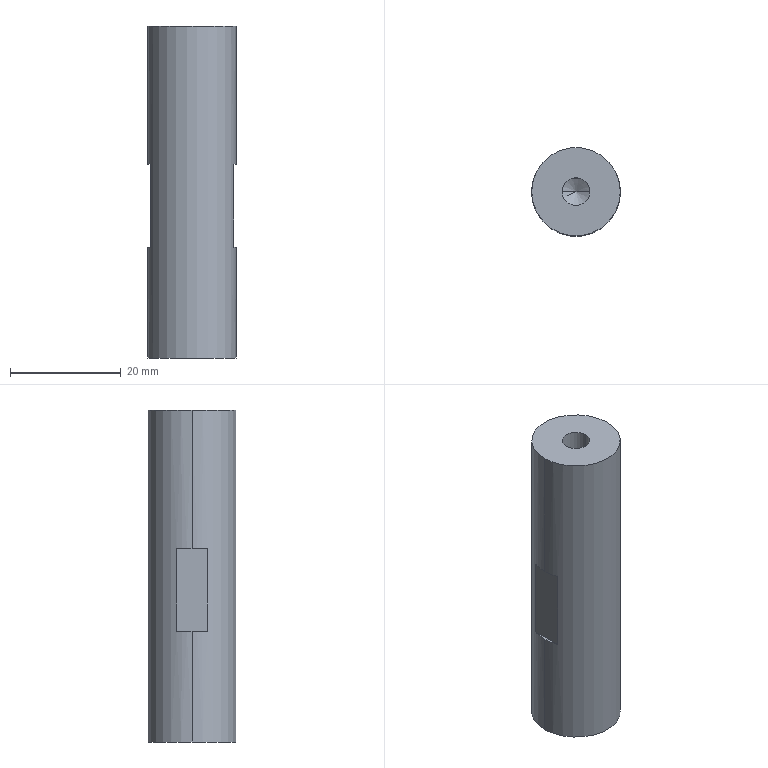Part | STEP file | detection post | 1 solid | 18 faces | box 16 x 16 x 60 mm | volume 11399 mm3 | plane 8 | cylinder 6 | cone 4 | commonest cylinder face diameters 5 x4 16 x2
STEP:
#1=CARTESIAN_POINT('',(0.,0.,0.));
#2=DIRECTION('',(0.,0.,1.));
#3=DIRECTION('',(1.,0.,0.));
#4=AXIS2_PLACEMENT_3D('',#1,#2,#3);
#5=CARTESIAN_POINT('',(2.5,0.,45.));
#6=VERTEX_POINT('',#5);
#7=CARTESIAN_POINT('',(2.5,0.,60.));
#8=VERTEX_POINT('',#7);
#9=CARTESIAN_POINT('',(2.5,0.,60.));
#10=DIRECTION('',(0.,0.,1.));
#11=VECTOR('',#10,1.);
#12=LINE('',#9,#11);
#13=CARTESIAN_POINT('',(0.,0.,60.));
#14=DIRECTION('',(0.,0.,1.));
#15=DIRECTION('',(1.,0.,0.));
#16=AXIS2_PLACEMENT_3D('',#13,#14,#15);
#17=CYLINDRICAL_SURFACE('',#16,2.5);
#18=CARTESIAN_POINT('',(6.283,0.));
#19=DIRECTION('',(0.,1.));
#20=VECTOR('',#19,1.);
#21=LINE('',#18,#20);
#22=(GEOMETRIC_REPRESENTATION_CONTEXT(2)PARAMETRIC_REPRESENTATION_CONTEXT()REPRESENTATION_CONTEXT('',''));
#23=DEFINITIONAL_REPRESENTATION('',(#21),#22);
#24=PCURVE('',#17,#23);
#25=CARTESIAN_POINT('',(0.,0.,60.));
#26=DIRECTION('',(0.,0.,1.));
#27=DIRECTION('',(1.,0.,0.));
#28=AXIS2_PLACEMENT_3D('',#25,#26,#27);
#29=CYLINDRICAL_SURFACE('',#28,2.5);
#30=CARTESIAN_POINT('',(0.,0.));
#31=DIRECTION('',(0.,1.));
#32=VECTOR('',#31,1.);
#33=LINE('',#30,#32);
#34=(GEOMETRIC_REPRESENTATION_CONTEXT(2)PARAMETRIC_REPRESENTATION_CONTEXT()REPRESENTATION_CONTEXT('',''));
#35=DEFINITIONAL_REPRESENTATION('',(#33),#34);
#36=PCURVE('',#29,#35);
#37=SURFACE_CURVE('',#12,(#24,#36),.PCURVE_S1.);
#38=EDGE_CURVE('',#6,#8,#37,.T.);
#39=ORIENTED_EDGE('',*,*,#38,.T.);
#40=CARTESIAN_POINT('',(-2.5,0.,60.));
#41=VERTEX_POINT('',#40);
#42=CARTESIAN_POINT('',(0.,0.,60.));
#43=DIRECTION('',(0.,0.,1.));
#44=DIRECTION('',(1.,0.,0.));
#45=AXIS2_PLACEMENT_3D('',#42,#43,#44);
#46=CIRCLE('',#45,2.5);
#47=CARTESIAN_POINT('',(0.,0.));
#48=DIRECTION('',(1.,0.));
#49=VECTOR('',#48,1.);
#50=LINE('',#47,#49);
#51=(GEOMETRIC_REPRESENTATION_CONTEXT(2)PARAMETRIC_REPRESENTATION_CONTEXT()REPRESENTATION_CONTEXT('',''));
#52=DEFINITIONAL_REPRESENTATION('',(#50),#51);
#53=PCURVE('',#17,#52);
#54=CARTESIAN_POINT('',(0.,0.,60.));
#55=DIRECTION('',(0.,0.,1.));
#56=DIRECTION('',(1.,0.,0.));
#57=AXIS2_PLACEMENT_3D('',#54,#55,#56);
#58=PLANE('',#57);
#59=CARTESIAN_POINT('',(0.,0.));
#60=DIRECTION('',(1.,0.));
#61=AXIS2_PLACEMENT_2D('',#59,#60);
#62=CIRCLE('',#61,2.5);
#63=(GEOMETRIC_REPRESENTATION_CONTEXT(2)PARAMETRIC_REPRESENTATION_CONTEXT()REPRESENTATION_CONTEXT('',''));
#64=DEFINITIONAL_REPRESENTATION('',(#62),#63);
#65=PCURVE('',#58,#64);
#66=SURFACE_CURVE('',#46,(#53,#65),.PCURVE_S1.);
#67=EDGE_CURVE('',#41,#8,#66,.T.);
#68=ORIENTED_EDGE('',*,*,#67,.F.);
#69=CARTESIAN_POINT('',(-2.5,0.,45.));
#70=VERTEX_POINT('',#69);
#71=CARTESIAN_POINT('',(-2.5,0.,60.));
#72=DIRECTION('',(0.,0.,1.));
#73=VECTOR('',#72,1.);
#74=LINE('',#71,#73);
#75=CARTESIAN_POINT('',(3.142,0.));
#76=DIRECTION('',(0.,1.));
#77=VECTOR('',#76,1.);
#78=LINE('',#75,#77);
#79=(GEOMETRIC_REPRESENTATION_CONTEXT(2)PARAMETRIC_REPRESENTATION_CONTEXT()REPRESENTATION_CONTEXT('',''));
#80=DEFINITIONAL_REPRESENTATION('',(#78),#79);
#81=PCURVE('',#17,#80);
#82=CARTESIAN_POINT('',(3.142,0.));
#83=DIRECTION('',(0.,1.));
#84=VECTOR('',#83,1.);
#85=LINE('',#82,#84);
#86=(GEOMETRIC_REPRESENTATION_CONTEXT(2)PARAMETRIC_REPRESENTATION_CONTEXT()REPRESENTATION_CONTEXT('',''));
#87=DEFINITIONAL_REPRESENTATION('',(#85),#86);
#88=PCURVE('',#29,#87);
#89=SURFACE_CURVE('',#74,(#81,#88),.PCURVE_S1.);
#90=EDGE_CURVE('',#70,#41,#89,.T.);
#91=ORIENTED_EDGE('',*,*,#90,.F.);
#92=CARTESIAN_POINT('',(0.,0.,45.));
#93=DIRECTION('',(0.,0.,1.));
#94=DIRECTION('',(1.,0.,0.));
#95=AXIS2_PLACEMENT_3D('',#92,#93,#94);
#96=CIRCLE('',#95,2.5);
#97=CARTESIAN_POINT('',(0.,-15.));
#98=DIRECTION('',(1.,0.));
#99=VECTOR('',#98,1.);
#100=LINE('',#97,#99);
#101=(GEOMETRIC_REPRESENTATION_CONTEXT(2)PARAMETRIC_REPRESENTATION_CONTEXT()REPRESENTATION_CONTEXT('',''));
#102=DEFINITIONAL_REPRESENTATION('',(#100),#101);
#103=PCURVE('',#17,#102);
#104=CARTESIAN_POINT('',(0.,0.,45.));
#105=DIRECTION('',(0.,0.,1.));
#106=DIRECTION('',(1.,0.,0.));
#107=AXIS2_PLACEMENT_3D('',#104,#105,#106);
#108=CONICAL_SURFACE('',#107,2.5,1.03);
#109=CARTESIAN_POINT('',(0.,0.));
#110=DIRECTION('',(1.,0.));
#111=VECTOR('',#110,1.);
#112=LINE('',#109,#111);
#113=(GEOMETRIC_REPRESENTATION_CONTEXT(2)PARAMETRIC_REPRESENTATION_CONTEXT()REPRESENTATION_CONTEXT('',''));
#114=DEFINITIONAL_REPRESENTATION('',(#112),#113);
#115=PCURVE('',#108,#114);
#116=SURFACE_CURVE('',#96,(#103,#115),.PCURVE_S1.);
#117=EDGE_CURVE('',#70,#6,#116,.T.);
#118=ORIENTED_EDGE('',*,*,#117,.T.);
#119=EDGE_LOOP('',(#39,#68,#91,#118));
#120=FACE_BOUND('',#119,.F.);
#121=ADVANCED_FACE('',(#120),#17,.F.);
#122=ORIENTED_EDGE('',*,*,#117,.F.);
#123=CARTESIAN_POINT('',(0.,0.,43.498));
#124=VERTEX_POINT('',#123);
#125=CARTESIAN_POINT('',(-2.5,0.,45.));
#126=DIRECTION('',(-0.8572,0.,0.515));
#127=VECTOR('',#126,1.);
#128=LINE('',#125,#127);
#129=CARTESIAN_POINT('',(3.142,0.));
#130=DIRECTION('',(0.,1.));
#131=VECTOR('',#130,1.);
#132=LINE('',#129,#131);
#133=(GEOMETRIC_REPRESENTATION_CONTEXT(2)PARAMETRIC_REPRESENTATION_CONTEXT()REPRESENTATION_CONTEXT('',''));
#134=DEFINITIONAL_REPRESENTATION('',(#132),#133);
#135=PCURVE('',#108,#134);
#136=CARTESIAN_POINT('',(0.,0.,45.));
#137=DIRECTION('',(0.,0.,1.));
#138=DIRECTION('',(1.,0.,0.));
#139=AXIS2_PLACEMENT_3D('',#136,#137,#138);
#140=CONICAL_SURFACE('',#139,2.5,1.03);
#141=CARTESIAN_POINT('',(3.142,0.));
#142=DIRECTION('',(0.,1.));
#143=VECTOR('',#142,1.);
#144=LINE('',#141,#143);
#145=(GEOMETRIC_REPRESENTATION_CONTEXT(2)PARAMETRIC_REPRESENTATION_CONTEXT()REPRESENTATION_CONTEXT('',''));
#146=DEFINITIONAL_REPRESENTATION('',(#144),#145);
#147=PCURVE('',#140,#146);
#148=SURFACE_CURVE('',#128,(#135,#147),.PCURVE_S1.);
#149=EDGE_CURVE('',#124,#70,#148,.T.);
#150=ORIENTED_EDGE('',*,*,#149,.F.);
#151=CARTESIAN_POINT('',(2.5,0.,45.));
#152=DIRECTION('',(0.8572,0.,0.515));
#153=VECTOR('',#152,1.);
#154=LINE('',#151,#153);
#155=CARTESIAN_POINT('',(6.283,0.));
#156=DIRECTION('',(0.,1.));
#157=VECTOR('',#156,1.);
#158=LINE('',#155,#157);
#159=(GEOMETRIC_REPRESENTATION_CONTEXT(2)PARAMETRIC_REPRESENTATION_CONTEXT()REPRESENTATION_CONTEXT('',''));
#160=DEFINITIONAL_REPRESENTATION('',(#158),#159);
#161=PCURVE('',#108,#160);
#162=CARTESIAN_POINT('',(0.,0.));
#163=DIRECTION('',(0.,1.));
#164=VECTOR('',#163,1.);
#165=LINE('',#162,#164);
#166=(GEOMETRIC_REPRESENTATION_CONTEXT(2)PARAMETRIC_REPRESENTATION_CONTEXT()REPRESENTATION_CONTEXT('',''));
#167=DEFINITIONAL_REPRESENTATION('',(#165),#166);
#168=PCURVE('',#140,#167);
#169=SURFACE_CURVE('',#154,(#161,#168),.PCURVE_S1.);
#170=EDGE_CURVE('',#124,#6,#169,.T.);
#171=ORIENTED_EDGE('',*,*,#170,.T.);
#172=EDGE_LOOP('',(#122,#150,#171));
#173=FACE_BOUND('',#172,.F.);
#174=ADVANCED_FACE('',(#173),#108,.F.);
#175=CARTESIAN_POINT('',(-2.5,0.,15.));
#176=VERTEX_POINT('',#175);
#177=CARTESIAN_POINT('',(-2.5,0.,0.));
#178=VERTEX_POINT('',#177);
#179=CARTESIAN_POINT('',(-2.5,0.,0.));
#180=DIRECTION('',(0.,0.,-1.));
#181=VECTOR('',#180,1.);
#182=LINE('',#179,#181);
#183=CARTESIAN_POINT('',(0.,0.,0.));
#184=DIRECTION('',(0.,0.,-1.));
#185=DIRECTION('',(-1.,0.,0.));
#186=AXIS2_PLACEMENT_3D('',#183,#184,#185);
#187=CYLINDRICAL_SURFACE('',#186,2.5);
#188=CARTESIAN_POINT('',(6.283,0.));
#189=DIRECTION('',(0.,1.));
#190=VECTOR('',#189,1.);
#191=LINE('',#188,#190);
#192=(GEOMETRIC_REPRESENTATION_CONTEXT(2)PARAMETRIC_REPRESENTATION_CONTEXT()REPRESENTATION_CONTEXT('',''));
#193=DEFINITIONAL_REPRESENTATION('',(#191),#192);
#194=PCURVE('',#187,#193);
#195=CARTESIAN_POINT('',(0.,0.,0.));
#196=DIRECTION('',(0.,0.,-1.));
#197=DIRECTION('',(-1.,0.,0.));
#198=AXIS2_PLACEMENT_3D('',#195,#196,#197);
#199=CYLINDRICAL_SURFACE('',#198,2.5);
#200=CARTESIAN_POINT('',(0.,0.));
#201=DIRECTION('',(0.,1.));
#202=VECTOR('',#201,1.);
#203=LINE('',#200,#202);
#204=(GEOMETRIC_REPRESENTATION_CONTEXT(2)PARAMETRIC_REPRESENTATION_CONTEXT()REPRESENTATION_CONTEXT('',''));
#205=DEFINITIONAL_REPRESENTATION('',(#203),#204);
#206=PCURVE('',#199,#205);
#207=SURFACE_CURVE('',#182,(#194,#206),.PCURVE_S1.);
#208=EDGE_CURVE('',#176,#178,#207,.T.);
#209=ORIENTED_EDGE('',*,*,#208,.T.);
#210=CARTESIAN_POINT('',(2.5,0.,0.));
#211=VERTEX_POINT('',#210);
#212=CARTESIAN_POINT('',(0.,0.,0.));
#213=DIRECTION('',(0.,0.,-1.));
#214=DIRECTION('',(-1.,0.,0.));
#215=AXIS2_PLACEMENT_3D('',#212,#213,#214);
#216=CIRCLE('',#215,2.5);
#217=CARTESIAN_POINT('',(0.,0.));
#218=DIRECTION('',(1.,0.));
#219=VECTOR('',#218,1.);
#220=LINE('',#217,#219);
#221=(GEOMETRIC_REPRESENTATION_CONTEXT(2)PARAMETRIC_REPRESENTATION_CONTEXT()REPRESENTATION_CONTEXT('',''));
#222=DEFINITIONAL_REPRESENTATION('',(#220),#221);
#223=PCURVE('',#187,#222);
#224=CARTESIAN_POINT('',(0.,0.,0.));
#225=DIRECTION('',(0.,0.,1.));
#226=DIRECTION('',(1.,0.,0.));
#227=AXIS2_PLACEMENT_3D('',#224,#225,#226);
#228=PLANE('',#227);
#229=CARTESIAN_POINT('',(-2.5,0.));
#230=CARTESIAN_POINT('',(-2.5,4.33));
#231=CARTESIAN_POINT('',(1.25,2.165));
#232=CARTESIAN_POINT('',(5.,0.));
#233=CARTESIAN_POINT('',(1.25,-2.165));
#234=CARTESIAN_POINT('',(-2.5,-4.33));
#235=CARTESIAN_POINT('',(-2.5,0.));
#236=(BOUNDED_CURVE()B_SPLINE_CURVE(2,(#229,#230,#231,#232,#233,#234,#235),.UNSPECIFIED.,.T.,.F.)B_SPLINE_CURVE_WITH_KNOTS((1,2,2,2,2,1),(-2.094,0.,2.094,4.189,6.283,8.378),.UNSPECIFIED.)CURVE()GEOMETRIC_REPRESENTATION_ITEM()RATIONAL_B_SPLINE_CURVE((1.,0.5,1.,0.5,1.,0.5,1.))REPRESENTATION_ITEM(''));
#237=(GEOMETRIC_REPRESENTATION_CONTEXT(2)PARAMETRIC_REPRESENTATION_CONTEXT()REPRESENTATION_CONTEXT('',''));
#238=DEFINITIONAL_REPRESENTATION('',(#236),#237);
#239=PCURVE('',#228,#238);
#240=SURFACE_CURVE('',#216,(#223,#239),.PCURVE_S1.);
#241=EDGE_CURVE('',#211,#178,#240,.T.);
#242=ORIENTED_EDGE('',*,*,#241,.F.);
#243=CARTESIAN_POINT('',(2.5,0.,15.));
#244=VERTEX_POINT('',#243);
#245=CARTESIAN_POINT('',(2.5,0.,0.));
#246=DIRECTION('',(0.,0.,-1.));
#247=VECTOR('',#246,1.);
#248=LINE('',#245,#247);
#249=CARTESIAN_POINT('',(3.142,0.));
#250=DIRECTION('',(0.,1.));
#251=VECTOR('',#250,1.);
#252=LINE('',#249,#251);
#253=(GEOMETRIC_REPRESENTATION_CONTEXT(2)PARAMETRIC_REPRESENTATION_CONTEXT()REPRESENTATION_CONTEXT('',''));
#254=DEFINITIONAL_REPRESENTATION('',(#252),#253);
#255=PCURVE('',#187,#254);
#256=CARTESIAN_POINT('',(3.142,0.));
#257=DIRECTION('',(0.,1.));
#258=VECTOR('',#257,1.);
#259=LINE('',#256,#258);
#260=(GEOMETRIC_REPRESENTATION_CONTEXT(2)PARAMETRIC_REPRESENTATION_CONTEXT()REPRESENTATION_CONTEXT('',''));
#261=DEFINITIONAL_REPRESENTATION('',(#259),#260);
#262=PCURVE('',#199,#261);
#263=SURFACE_CURVE('',#248,(#255,#262),.PCURVE_S1.);
#264=EDGE_CURVE('',#244,#211,#263,.T.);
#265=ORIENTED_EDGE('',*,*,#264,.F.);
#266=CARTESIAN_POINT('',(0.,0.,15.));
#267=DIRECTION('',(0.,0.,-1.));
#268=DIRECTION('',(-1.,0.,0.));
#269=AXIS2_PLACEMENT_3D('',#266,#267,#268);
#270=CIRCLE('',#269,2.5);
#271=CARTESIAN_POINT('',(0.,-15.));
#272=DIRECTION('',(1.,0.));
#273=VECTOR('',#272,1.);
#274=LINE('',#271,#273);
#275=(GEOMETRIC_REPRESENTATION_CONTEXT(2)PARAMETRIC_REPRESENTATION_CONTEXT()REPRESENTATION_CONTEXT('',''));
#276=DEFINITIONAL_REPRESENTATION('',(#274),#275);
#277=PCURVE('',#187,#276);
#278=CARTESIAN_POINT('',(0.,0.,15.));
#279=DIRECTION('',(0.,0.,-1.));
#280=DIRECTION('',(-1.,0.,0.));
#281=AXIS2_PLACEMENT_3D('',#278,#279,#280);
#282=CONICAL_SURFACE('',#281,2.5,1.03);
#283=CARTESIAN_POINT('',(0.,0.));
#284=DIRECTION('',(1.,0.));
#285=VECTOR('',#284,1.);
#286=LINE('',#283,#285);
#287=(GEOMETRIC_REPRESENTATION_CONTEXT(2)PARAMETRIC_REPRESENTATION_CONTEXT()REPRESENTATION_CONTEXT('',''));
#288=DEFINITIONAL_REPRESENTATION('',(#286),#287);
#289=PCURVE('',#282,#288);
#290=SURFACE_CURVE('',#270,(#277,#289),.PCURVE_S1.);
#291=EDGE_CURVE('',#244,#176,#290,.T.);
#292=ORIENTED_EDGE('',*,*,#291,.T.);
#293=EDGE_LOOP('',(#209,#242,#265,#292));
#294=FACE_BOUND('',#293,.F.);
#295=ADVANCED_FACE('',(#294),#187,.F.);
#296=ORIENTED_EDGE('',*,*,#291,.F.);
#297=CARTESIAN_POINT('',(0.,0.,16.502));
#298=VERTEX_POINT('',#297);
#299=CARTESIAN_POINT('',(2.5,0.,15.));
#300=DIRECTION('',(0.8572,0.,-0.515));
#301=VECTOR('',#300,1.);
#302=LINE('',#299,#301);
#303=CARTESIAN_POINT('',(3.142,0.));
#304=DIRECTION('',(0.,1.));
#305=VECTOR('',#304,1.);
#306=LINE('',#303,#305);
#307=(GEOMETRIC_REPRESENTATION_CONTEXT(2)PARAMETRIC_REPRESENTATION_CONTEXT()REPRESENTATION_CONTEXT('',''));
#308=DEFINITIONAL_REPRESENTATION('',(#306),#307);
#309=PCURVE('',#282,#308);
#310=CARTESIAN_POINT('',(0.,0.,15.));
#311=DIRECTION('',(0.,0.,-1.));
#312=DIRECTION('',(-1.,0.,0.));
#313=AXIS2_PLACEMENT_3D('',#310,#311,#312);
#314=CONICAL_SURFACE('',#313,2.5,1.03);
#315=CARTESIAN_POINT('',(3.142,0.));
#316=DIRECTION('',(0.,1.));
#317=VECTOR('',#316,1.);
#318=LINE('',#315,#317);
#319=(GEOMETRIC_REPRESENTATION_CONTEXT(2)PARAMETRIC_REPRESENTATION_CONTEXT()REPRESENTATION_CONTEXT('',''));
#320=DEFINITIONAL_REPRESENTATION('',(#318),#319);
#321=PCURVE('',#314,#320);
#322=SURFACE_CURVE('',#302,(#309,#321),.PCURVE_S1.);
#323=EDGE_CURVE('',#298,#244,#322,.T.);
#324=ORIENTED_EDGE('',*,*,#323,.F.);
#325=CARTESIAN_POINT('',(-2.5,0.,15.));
#326=DIRECTION('',(-0.8572,0.,-0.515));
#327=VECTOR('',#326,1.);
#328=LINE('',#325,#327);
#329=CARTESIAN_POINT('',(6.283,0.));
#330=DIRECTION('',(0.,1.));
#331=VECTOR('',#330,1.);
#332=LINE('',#329,#331);
#333=(GEOMETRIC_REPRESENTATION_CONTEXT(2)PARAMETRIC_REPRESENTATION_CONTEXT()REPRESENTATION_CONTEXT('',''));
#334=DEFINITIONAL_REPRESENTATION('',(#332),#333);
#335=PCURVE('',#282,#334);
#336=CARTESIAN_POINT('',(0.,0.));
#337=DIRECTION('',(0.,1.));
#338=VECTOR('',#337,1.);
#339=LINE('',#336,#338);
#340=(GEOMETRIC_REPRESENTATION_CONTEXT(2)PARAMETRIC_REPRESENTATION_CONTEXT()REPRESENTATION_CONTEXT('',''));
#341=DEFINITIONAL_REPRESENTATION('',(#339),#340);
#342=PCURVE('',#314,#341);
#343=SURFACE_CURVE('',#328,(#335,#342),.PCURVE_S1.);
#344=EDGE_CURVE('',#298,#176,#343,.T.);
#345=ORIENTED_EDGE('',*,*,#344,.T.);
#346=EDGE_LOOP('',(#296,#324,#345));
#347=FACE_BOUND('',#346,.F.);
#348=ADVANCED_FACE('',(#347),#282,.F.);
#349=CARTESIAN_POINT('',(8.,0.,60.));
#350=VERTEX_POINT('',#349);
#351=CARTESIAN_POINT('',(-8.,0.,60.));
#352=VERTEX_POINT('',#351);
#353=CARTESIAN_POINT('',(0.,0.,60.));
#354=DIRECTION('',(0.,0.,1.));
#355=DIRECTION('',(1.,0.,0.));
#356=AXIS2_PLACEMENT_3D('',#353,#354,#355);
#357=CIRCLE('',#356,8.);
#358=CARTESIAN_POINT('',(0.,0.,60.));
#359=DIRECTION('',(0.,0.,-1.));
#360=DIRECTION('',(-1.,0.,0.));
#361=AXIS2_PLACEMENT_3D('',#358,#359,#360);
#362=CYLINDRICAL_SURFACE('',#361,8.);
#363=CARTESIAN_POINT('',(3.142,0.));
#364=DIRECTION('',(-1.,0.));
#365=VECTOR('',#364,1.);
#366=LINE('',#363,#365);
#367=(GEOMETRIC_REPRESENTATION_CONTEXT(2)PARAMETRIC_REPRESENTATION_CONTEXT()REPRESENTATION_CONTEXT('',''));
#368=DEFINITIONAL_REPRESENTATION('',(#366),#367);
#369=PCURVE('',#362,#368);
#370=CARTESIAN_POINT('',(0.,0.));
#371=DIRECTION('',(1.,0.));
#372=AXIS2_PLACEMENT_2D('',#370,#371);
#373=CIRCLE('',#372,8.);
#374=(GEOMETRIC_REPRESENTATION_CONTEXT(2)PARAMETRIC_REPRESENTATION_CONTEXT()REPRESENTATION_CONTEXT('',''));
#375=DEFINITIONAL_REPRESENTATION('',(#373),#374);
#376=PCURVE('',#58,#375);
#377=SURFACE_CURVE('',#357,(#369,#376),.PCURVE_S1.);
#378=EDGE_CURVE('',#350,#352,#377,.T.);
#379=ORIENTED_EDGE('',*,*,#378,.F.);
#380=CARTESIAN_POINT('',(8.,0.,35.));
#381=VERTEX_POINT('',#380);
#382=CARTESIAN_POINT('',(8.,0.,60.));
#383=DIRECTION('',(0.,0.,-1.));
#384=VECTOR('',#383,1.);
#385=LINE('',#382,#384);
#386=CARTESIAN_POINT('',(3.142,0.));
#387=DIRECTION('',(0.,1.));
#388=VECTOR('',#387,1.);
#389=LINE('',#386,#388);
#390=(GEOMETRIC_REPRESENTATION_CONTEXT(2)PARAMETRIC_REPRESENTATION_CONTEXT()REPRESENTATION_CONTEXT('',''));
#391=DEFINITIONAL_REPRESENTATION('',(#389),#390);
#392=PCURVE('',#362,#391);
#393=CARTESIAN_POINT('',(0.,0.,60.));
#394=DIRECTION('',(0.,0.,-1.));
#395=DIRECTION('',(-1.,0.,0.));
#396=AXIS2_PLACEMENT_3D('',#393,#394,#395);
#397=CYLINDRICAL_SURFACE('',#396,8.);
#398=CARTESIAN_POINT('',(3.142,0.));
#399=DIRECTION('',(0.,1.));
#400=VECTOR('',#399,1.);
#401=LINE('',#398,#400);
#402=(GEOMETRIC_REPRESENTATION_CONTEXT(2)PARAMETRIC_REPRESENTATION_CONTEXT()REPRESENTATION_CONTEXT('',''));
#403=DEFINITIONAL_REPRESENTATION('',(#401),#402);
#404=PCURVE('',#397,#403);
#405=SURFACE_CURVE('',#385,(#392,#404),.PCURVE_S1.);
#406=EDGE_CURVE('',#350,#381,#405,.T.);
#407=ORIENTED_EDGE('',*,*,#406,.T.);
#408=CARTESIAN_POINT('',(7.5,2.784,35.));
#409=VERTEX_POINT('',#408);
#410=CARTESIAN_POINT('',(0.,0.,35.));
#411=DIRECTION('',(0.,0.,-1.));
#412=DIRECTION('',(-1.,0.,0.));
#413=AXIS2_PLACEMENT_3D('',#410,#411,#412);
#414=CIRCLE('',#413,8.);
#415=CARTESIAN_POINT('',(0.,25.));
#416=DIRECTION('',(1.,0.));
#417=VECTOR('',#416,1.);
#418=LINE('',#415,#417);
#419=(GEOMETRIC_REPRESENTATION_CONTEXT(2)PARAMETRIC_REPRESENTATION_CONTEXT()REPRESENTATION_CONTEXT('',''));
#420=DEFINITIONAL_REPRESENTATION('',(#418),#419);
#421=PCURVE('',#362,#420);
#422=CARTESIAN_POINT('',(7.5,91.25,35.));
#423=DIRECTION('',(0.,0.,-1.));
#424=DIRECTION('',(-1.,0.,0.));
#425=AXIS2_PLACEMENT_3D('',#422,#423,#424);
#426=PLANE('',#425);
#427=CARTESIAN_POINT('',(7.5,-91.25));
#428=DIRECTION('',(1.,0.));
#429=AXIS2_PLACEMENT_2D('',#427,#428);
#430=CIRCLE('',#429,8.);
#431=(GEOMETRIC_REPRESENTATION_CONTEXT(2)PARAMETRIC_REPRESENTATION_CONTEXT()REPRESENTATION_CONTEXT('',''));
#432=DEFINITIONAL_REPRESENTATION('',(#430),#431);
#433=PCURVE('',#426,#432);
#434=SURFACE_CURVE('',#414,(#421,#433),.PCURVE_S1.);
#435=EDGE_CURVE('',#409,#381,#434,.T.);
#436=ORIENTED_EDGE('',*,*,#435,.F.);
#437=CARTESIAN_POINT('',(7.5,2.784,20.));
#438=VERTEX_POINT('',#437);
#439=CARTESIAN_POINT('',(7.5,2.784,60.));
#440=DIRECTION('',(0.,0.,1.));
#441=VECTOR('',#440,1.);
#442=LINE('',#439,#441);
#443=CARTESIAN_POINT('',(2.786,0.));
#444=DIRECTION('',(0.,-1.));
#445=VECTOR('',#444,1.);
#446=LINE('',#443,#445);
#447=(GEOMETRIC_REPRESENTATION_CONTEXT(2)PARAMETRIC_REPRESENTATION_CONTEXT()REPRESENTATION_CONTEXT('',''));
#448=DEFINITIONAL_REPRESENTATION('',(#446),#447);
#449=PCURVE('',#362,#448);
#450=CARTESIAN_POINT('',(7.5,91.25,20.));
#451=DIRECTION('',(1.,0.,0.));
#452=DIRECTION('',(0.,0.,-1.));
#453=AXIS2_PLACEMENT_3D('',#450,#451,#452);
#454=PLANE('',#453);
#455=CARTESIAN_POINT('',(-40.,-88.466));
#456=DIRECTION('',(-1.,0.));
#457=VECTOR('',#456,1.);
#458=LINE('',#455,#457);
#459=(GEOMETRIC_REPRESENTATION_CONTEXT(2)PARAMETRIC_REPRESENTATION_CONTEXT()REPRESENTATION_CONTEXT('',''));
#460=DEFINITIONAL_REPRESENTATION('',(#458),#459);
#461=PCURVE('',#454,#460);
#462=SURFACE_CURVE('',#442,(#449,#461),.PCURVE_S1.);
#463=EDGE_CURVE('',#438,#409,#462,.T.);
#464=ORIENTED_EDGE('',*,*,#463,.F.);
#465=CARTESIAN_POINT('',(8.,0.,20.));
#466=VERTEX_POINT('',#465);
#467=CARTESIAN_POINT('',(0.,0.,20.));
#468=DIRECTION('',(0.,0.,1.));
#469=DIRECTION('',(1.,0.,0.));
#470=AXIS2_PLACEMENT_3D('',#467,#468,#469);
#471=CIRCLE('',#470,8.);
#472=CARTESIAN_POINT('',(3.142,40.));
#473=DIRECTION('',(-1.,0.));
#474=VECTOR('',#473,1.);
#475=LINE('',#472,#474);
#476=(GEOMETRIC_REPRESENTATION_CONTEXT(2)PARAMETRIC_REPRESENTATION_CONTEXT()REPRESENTATION_CONTEXT('',''));
#477=DEFINITIONAL_REPRESENTATION('',(#475),#476);
#478=PCURVE('',#362,#477);
#479=CARTESIAN_POINT('',(7.5,91.25,20.));
#480=DIRECTION('',(0.,0.,1.));
#481=DIRECTION('',(1.,0.,0.));
#482=AXIS2_PLACEMENT_3D('',#479,#480,#481);
#483=PLANE('',#482);
#484=CARTESIAN_POINT('',(-7.5,-91.25));
#485=DIRECTION('',(1.,0.));
#486=AXIS2_PLACEMENT_2D('',#484,#485);
#487=CIRCLE('',#486,8.);
#488=(GEOMETRIC_REPRESENTATION_CONTEXT(2)PARAMETRIC_REPRESENTATION_CONTEXT()REPRESENTATION_CONTEXT('',''));
#489=DEFINITIONAL_REPRESENTATION('',(#487),#488);
#490=PCURVE('',#483,#489);
#491=SURFACE_CURVE('',#471,(#478,#490),.PCURVE_S1.);
#492=EDGE_CURVE('',#466,#438,#491,.T.);
#493=ORIENTED_EDGE('',*,*,#492,.F.);
#494=CARTESIAN_POINT('',(8.,0.,0.));
#495=VERTEX_POINT('',#494);
#496=CARTESIAN_POINT('',(8.,0.,60.));
#497=DIRECTION('',(0.,0.,-1.));
#498=VECTOR('',#497,1.);
#499=LINE('',#496,#498);
#500=CARTESIAN_POINT('',(3.142,0.));
#501=DIRECTION('',(0.,1.));
#502=VECTOR('',#501,1.);
#503=LINE('',#500,#502);
#504=(GEOMETRIC_REPRESENTATION_CONTEXT(2)PARAMETRIC_REPRESENTATION_CONTEXT()REPRESENTATION_CONTEXT('',''));
#505=DEFINITIONAL_REPRESENTATION('',(#503),#504);
#506=PCURVE('',#362,#505);
#507=CARTESIAN_POINT('',(3.142,0.));
#508=DIRECTION('',(0.,1.));
#509=VECTOR('',#508,1.);
#510=LINE('',#507,#509);
#511=(GEOMETRIC_REPRESENTATION_CONTEXT(2)PARAMETRIC_REPRESENTATION_CONTEXT()REPRESENTATION_CONTEXT('',''));
#512=DEFINITIONAL_REPRESENTATION('',(#510),#511);
#513=PCURVE('',#397,#512);
#514=SURFACE_CURVE('',#499,(#506,#513),.PCURVE_S1.);
#515=EDGE_CURVE('',#466,#495,#514,.T.);
#516=ORIENTED_EDGE('',*,*,#515,.T.);
#517=CARTESIAN_POINT('',(-8.,0.,0.));
#518=VERTEX_POINT('',#517);
#519=CARTESIAN_POINT('',(0.,0.,0.));
#520=DIRECTION('',(0.,0.,1.));
#521=DIRECTION('',(1.,0.,0.));
#522=AXIS2_PLACEMENT_3D('',#519,#520,#521);
#523=CIRCLE('',#522,8.);
#524=CARTESIAN_POINT('',(3.142,60.));
#525=DIRECTION('',(-1.,0.));
#526=VECTOR('',#525,1.);
#527=LINE('',#524,#526);
#528=(GEOMETRIC_REPRESENTATION_CONTEXT(2)PARAMETRIC_REPRESENTATION_CONTEXT()REPRESENTATION_CONTEXT('',''));
#529=DEFINITIONAL_REPRESENTATION('',(#527),#528);
#530=PCURVE('',#362,#529);
#531=CARTESIAN_POINT('',(0.,0.));
#532=DIRECTION('',(1.,0.));
#533=AXIS2_PLACEMENT_2D('',#531,#532);
#534=CIRCLE('',#533,8.);
#535=(GEOMETRIC_REPRESENTATION_CONTEXT(2)PARAMETRIC_REPRESENTATION_CONTEXT()REPRESENTATION_CONTEXT('',''));
#536=DEFINITIONAL_REPRESENTATION('',(#534),#535);
#537=PCURVE('',#228,#536);
#538=SURFACE_CURVE('',#523,(#530,#537),.PCURVE_S1.);
#539=EDGE_CURVE('',#495,#518,#538,.T.);
#540=ORIENTED_EDGE('',*,*,#539,.T.);
#541=CARTESIAN_POINT('',(-8.,0.,20.));
#542=VERTEX_POINT('',#541);
#543=CARTESIAN_POINT('',(-8.,0.,60.));
#544=DIRECTION('',(0.,0.,-1.));
#545=VECTOR('',#544,1.);
#546=LINE('',#543,#545);
#547=CARTESIAN_POINT('',(0.,0.));
#548=DIRECTION('',(0.,1.));
#549=VECTOR('',#548,1.);
#550=LINE('',#547,#549);
#551=(GEOMETRIC_REPRESENTATION_CONTEXT(2)PARAMETRIC_REPRESENTATION_CONTEXT()REPRESENTATION_CONTEXT('',''));
#552=DEFINITIONAL_REPRESENTATION('',(#550),#551);
#553=PCURVE('',#362,#552);
#554=CARTESIAN_POINT('',(6.283,0.));
#555=DIRECTION('',(0.,1.));
#556=VECTOR('',#555,1.);
#557=LINE('',#554,#556);
#558=(GEOMETRIC_REPRESENTATION_CONTEXT(2)PARAMETRIC_REPRESENTATION_CONTEXT()REPRESENTATION_CONTEXT('',''));
#559=DEFINITIONAL_REPRESENTATION('',(#557),#558);
#560=PCURVE('',#397,#559);
#561=SURFACE_CURVE('',#546,(#553,#560),.PCURVE_S1.);
#562=EDGE_CURVE('',#542,#518,#561,.T.);
#563=ORIENTED_EDGE('',*,*,#562,.F.);
#564=CARTESIAN_POINT('',(-7.5,2.784,20.));
#565=VERTEX_POINT('',#564);
#566=CARTESIAN_POINT('',(0.,0.,20.));
#567=DIRECTION('',(0.,0.,1.));
#568=DIRECTION('',(1.,0.,0.));
#569=AXIS2_PLACEMENT_3D('',#566,#567,#568);
#570=CIRCLE('',#569,8.);
#571=CARTESIAN_POINT('',(3.142,40.));
#572=DIRECTION('',(-1.,0.));
#573=VECTOR('',#572,1.);
#574=LINE('',#571,#573);
#575=(GEOMETRIC_REPRESENTATION_CONTEXT(2)PARAMETRIC_REPRESENTATION_CONTEXT()REPRESENTATION_CONTEXT('',''));
#576=DEFINITIONAL_REPRESENTATION('',(#574),#575);
#577=PCURVE('',#362,#576);
#578=CARTESIAN_POINT('',(-17.514,91.25,20.));
#579=DIRECTION('',(0.,0.,1.));
#580=DIRECTION('',(1.,0.,0.));
#581=AXIS2_PLACEMENT_3D('',#578,#579,#580);
#582=PLANE('',#581);
#583=CARTESIAN_POINT('',(17.514,-91.25));
#584=DIRECTION('',(1.,0.));
#585=AXIS2_PLACEMENT_2D('',#583,#584);
#586=CIRCLE('',#585,8.);
#587=(GEOMETRIC_REPRESENTATION_CONTEXT(2)PARAMETRIC_REPRESENTATION_CONTEXT()REPRESENTATION_CONTEXT('',''));
#588=DEFINITIONAL_REPRESENTATION('',(#586),#587);
#589=PCURVE('',#582,#588);
#590=SURFACE_CURVE('',#570,(#577,#589),.PCURVE_S1.);
#591=EDGE_CURVE('',#565,#542,#590,.T.);
#592=ORIENTED_EDGE('',*,*,#591,.F.);
#593=CARTESIAN_POINT('',(-7.5,2.784,35.));
#594=VERTEX_POINT('',#593);
#595=CARTESIAN_POINT('',(-7.5,2.784,60.));
#596=DIRECTION('',(0.,0.,-1.));
#597=VECTOR('',#596,1.);
#598=LINE('',#595,#597);
#599=CARTESIAN_POINT('',(0.3554,0.));
#600=DIRECTION('',(0.,1.));
#601=VECTOR('',#600,1.);
#602=LINE('',#599,#601);
#603=(GEOMETRIC_REPRESENTATION_CONTEXT(2)PARAMETRIC_REPRESENTATION_CONTEXT()REPRESENTATION_CONTEXT('',''));
#604=DEFINITIONAL_REPRESENTATION('',(#602),#603);
#605=PCURVE('',#362,#604);
#606=CARTESIAN_POINT('',(-7.5,91.25,20.));
#607=DIRECTION('',(-1.,0.,0.));
#608=DIRECTION('',(0.,0.,1.));
#609=AXIS2_PLACEMENT_3D('',#606,#607,#608);
#610=PLANE('',#609);
#611=CARTESIAN_POINT('',(40.,-88.466));
#612=DIRECTION('',(-1.,0.));
#613=VECTOR('',#612,1.);
#614=LINE('',#611,#613);
#615=(GEOMETRIC_REPRESENTATION_CONTEXT(2)PARAMETRIC_REPRESENTATION_CONTEXT()REPRESENTATION_CONTEXT('',''));
#616=DEFINITIONAL_REPRESENTATION('',(#614),#615);
#617=PCURVE('',#610,#616);
#618=SURFACE_CURVE('',#598,(#605,#617),.PCURVE_S1.);
#619=EDGE_CURVE('',#594,#565,#618,.T.);
#620=ORIENTED_EDGE('',*,*,#619,.F.);
#621=CARTESIAN_POINT('',(-8.,0.,35.));
#622=VERTEX_POINT('',#621);
#623=CARTESIAN_POINT('',(0.,0.,35.));
#624=DIRECTION('',(0.,0.,-1.));
#625=DIRECTION('',(-1.,0.,0.));
#626=AXIS2_PLACEMENT_3D('',#623,#624,#625);
#627=CIRCLE('',#626,8.);
#628=CARTESIAN_POINT('',(0.,25.));
#629=DIRECTION('',(1.,0.));
#630=VECTOR('',#629,1.);
#631=LINE('',#628,#630);
#632=(GEOMETRIC_REPRESENTATION_CONTEXT(2)PARAMETRIC_REPRESENTATION_CONTEXT()REPRESENTATION_CONTEXT('',''));
#633=DEFINITIONAL_REPRESENTATION('',(#631),#632);
#634=PCURVE('',#362,#633);
#635=CARTESIAN_POINT('',(-17.514,91.25,35.));
#636=DIRECTION('',(0.,0.,-1.));
#637=DIRECTION('',(-1.,0.,0.));
#638=AXIS2_PLACEMENT_3D('',#635,#636,#637);
#639=PLANE('',#638);
#640=CARTESIAN_POINT('',(-17.514,-91.25));
#641=DIRECTION('',(1.,0.));
#642=AXIS2_PLACEMENT_2D('',#640,#641);
#643=CIRCLE('',#642,8.);
#644=(GEOMETRIC_REPRESENTATION_CONTEXT(2)PARAMETRIC_REPRESENTATION_CONTEXT()REPRESENTATION_CONTEXT('',''));
#645=DEFINITIONAL_REPRESENTATION('',(#643),#644);
#646=PCURVE('',#639,#645);
#647=SURFACE_CURVE('',#627,(#634,#646),.PCURVE_S1.);
#648=EDGE_CURVE('',#622,#594,#647,.T.);
#649=ORIENTED_EDGE('',*,*,#648,.F.);
#650=CARTESIAN_POINT('',(-8.,0.,60.));
#651=DIRECTION('',(0.,0.,-1.));
#652=VECTOR('',#651,1.);
#653=LINE('',#650,#652);
#654=CARTESIAN_POINT('',(0.,0.));
#655=DIRECTION('',(0.,1.));
#656=VECTOR('',#655,1.);
#657=LINE('',#654,#656);
#658=(GEOMETRIC_REPRESENTATION_CONTEXT(2)PARAMETRIC_REPRESENTATION_CONTEXT()REPRESENTATION_CONTEXT('',''));
#659=DEFINITIONAL_REPRESENTATION('',(#657),#658);
#660=PCURVE('',#362,#659);
#661=CARTESIAN_POINT('',(6.283,0.));
#662=DIRECTION('',(0.,1.));
#663=VECTOR('',#662,1.);
#664=LINE('',#661,#663);
#665=(GEOMETRIC_REPRESENTATION_CONTEXT(2)PARAMETRIC_REPRESENTATION_CONTEXT()REPRESENTATION_CONTEXT('',''));
#666=DEFINITIONAL_REPRESENTATION('',(#664),#665);
#667=PCURVE('',#397,#666);
#668=SURFACE_CURVE('',#653,(#660,#667),.PCURVE_S1.);
#669=EDGE_CURVE('',#352,#622,#668,.T.);
#670=ORIENTED_EDGE('',*,*,#669,.F.);
#671=EDGE_LOOP('',(#379,#407,#436,#464,#493,#516,#540,#563,#592,#620,#649,#670));
#672=FACE_BOUND('',#671,.T.);
#673=ADVANCED_FACE('',(#672),#362,.T.);
#674=ORIENTED_EDGE('',*,*,#406,.F.);
#675=CARTESIAN_POINT('',(0.,0.,60.));
#676=DIRECTION('',(0.,0.,1.));
#677=DIRECTION('',(1.,0.,0.));
#678=AXIS2_PLACEMENT_3D('',#675,#676,#677);
#679=CIRCLE('',#678,8.);
#680=CARTESIAN_POINT('',(9.425,0.));
#681=DIRECTION('',(-1.,0.));
#682=VECTOR('',#681,1.);
#683=LINE('',#680,#682);
#684=(GEOMETRIC_REPRESENTATION_CONTEXT(2)PARAMETRIC_REPRESENTATION_CONTEXT()REPRESENTATION_CONTEXT('',''));
#685=DEFINITIONAL_REPRESENTATION('',(#683),#684);
#686=PCURVE('',#397,#685);
#687=CARTESIAN_POINT('',(0.,0.));
#688=DIRECTION('',(1.,0.));
#689=AXIS2_PLACEMENT_2D('',#687,#688);
#690=CIRCLE('',#689,8.);
#691=(GEOMETRIC_REPRESENTATION_CONTEXT(2)PARAMETRIC_REPRESENTATION_CONTEXT()REPRESENTATION_CONTEXT('',''));
#692=DEFINITIONAL_REPRESENTATION('',(#690),#691);
#693=PCURVE('',#58,#692);
#694=SURFACE_CURVE('',#679,(#686,#693),.PCURVE_S1.);
#695=EDGE_CURVE('',#352,#350,#694,.T.);
#696=ORIENTED_EDGE('',*,*,#695,.F.);
#697=ORIENTED_EDGE('',*,*,#669,.T.);
#698=CARTESIAN_POINT('',(-7.5,-2.784,35.));
#699=VERTEX_POINT('',#698);
#700=CARTESIAN_POINT('',(0.,0.,35.));
#701=DIRECTION('',(0.,0.,-1.));
#702=DIRECTION('',(-1.,0.,0.));
#703=AXIS2_PLACEMENT_3D('',#700,#701,#702);
#704=CIRCLE('',#703,8.);
#705=CARTESIAN_POINT('',(0.,25.));
#706=DIRECTION('',(1.,0.));
#707=VECTOR('',#706,1.);
#708=LINE('',#705,#707);
#709=(GEOMETRIC_REPRESENTATION_CONTEXT(2)PARAMETRIC_REPRESENTATION_CONTEXT()REPRESENTATION_CONTEXT('',''));
#710=DEFINITIONAL_REPRESENTATION('',(#708),#709);
#711=PCURVE('',#397,#710);
#712=CARTESIAN_POINT('',(-17.514,-91.25));
#713=DIRECTION('',(1.,0.));
#714=AXIS2_PLACEMENT_2D('',#712,#713);
#715=CIRCLE('',#714,8.);
#716=(GEOMETRIC_REPRESENTATION_CONTEXT(2)PARAMETRIC_REPRESENTATION_CONTEXT()REPRESENTATION_CONTEXT('',''));
#717=DEFINITIONAL_REPRESENTATION('',(#715),#716);
#718=PCURVE('',#639,#717);
#719=SURFACE_CURVE('',#704,(#711,#718),.PCURVE_S1.);
#720=EDGE_CURVE('',#699,#622,#719,.T.);
#721=ORIENTED_EDGE('',*,*,#720,.F.);
#722=CARTESIAN_POINT('',(-7.5,-2.784,20.));
#723=VERTEX_POINT('',#722);
#724=CARTESIAN_POINT('',(-7.5,-2.784,60.));
#725=DIRECTION('',(0.,0.,1.));
#726=VECTOR('',#725,1.);
#727=LINE('',#724,#726);
#728=CARTESIAN_POINT('',(5.928,0.));
#729=DIRECTION('',(0.,-1.));
#730=VECTOR('',#729,1.);
#731=LINE('',#728,#730);
#732=(GEOMETRIC_REPRESENTATION_CONTEXT(2)PARAMETRIC_REPRESENTATION_CONTEXT()REPRESENTATION_CONTEXT('',''));
#733=DEFINITIONAL_REPRESENTATION('',(#731),#732);
#734=PCURVE('',#397,#733);
#735=CARTESIAN_POINT('',(40.,-94.034));
#736=DIRECTION('',(1.,0.));
#737=VECTOR('',#736,1.);
#738=LINE('',#735,#737);
#739=(GEOMETRIC_REPRESENTATION_CONTEXT(2)PARAMETRIC_REPRESENTATION_CONTEXT()REPRESENTATION_CONTEXT('',''));
#740=DEFINITIONAL_REPRESENTATION('',(#738),#739);
#741=PCURVE('',#610,#740);
#742=SURFACE_CURVE('',#727,(#734,#741),.PCURVE_S1.);
#743=EDGE_CURVE('',#723,#699,#742,.T.);
#744=ORIENTED_EDGE('',*,*,#743,.F.);
#745=CARTESIAN_POINT('',(0.,0.,20.));
#746=DIRECTION('',(0.,0.,1.));
#747=DIRECTION('',(1.,0.,0.));
#748=AXIS2_PLACEMENT_3D('',#745,#746,#747);
#749=CIRCLE('',#748,8.);
#750=CARTESIAN_POINT('',(9.425,40.));
#751=DIRECTION('',(-1.,0.));
#752=VECTOR('',#751,1.);
#753=LINE('',#750,#752);
#754=(GEOMETRIC_REPRESENTATION_CONTEXT(2)PARAMETRIC_REPRESENTATION_CONTEXT()REPRESENTATION_CONTEXT('',''));
#755=DEFINITIONAL_REPRESENTATION('',(#753),#754);
#756=PCURVE('',#397,#755);
#757=CARTESIAN_POINT('',(17.514,-91.25));
#758=DIRECTION('',(1.,0.));
#759=AXIS2_PLACEMENT_2D('',#757,#758);
#760=CIRCLE('',#759,8.);
#761=(GEOMETRIC_REPRESENTATION_CONTEXT(2)PARAMETRIC_REPRESENTATION_CONTEXT()REPRESENTATION_CONTEXT('',''));
#762=DEFINITIONAL_REPRESENTATION('',(#760),#761);
#763=PCURVE('',#582,#762);
#764=SURFACE_CURVE('',#749,(#756,#763),.PCURVE_S1.);
#765=EDGE_CURVE('',#542,#723,#764,.T.);
#766=ORIENTED_EDGE('',*,*,#765,.F.);
#767=ORIENTED_EDGE('',*,*,#562,.T.);
#768=CARTESIAN_POINT('',(0.,0.,0.));
#769=DIRECTION('',(0.,0.,1.));
#770=DIRECTION('',(1.,0.,0.));
#771=AXIS2_PLACEMENT_3D('',#768,#769,#770);
#772=CIRCLE('',#771,8.);
#773=CARTESIAN_POINT('',(9.425,60.));
#774=DIRECTION('',(-1.,0.));
#775=VECTOR('',#774,1.);
#776=LINE('',#773,#775);
#777=(GEOMETRIC_REPRESENTATION_CONTEXT(2)PARAMETRIC_REPRESENTATION_CONTEXT()REPRESENTATION_CONTEXT('',''));
#778=DEFINITIONAL_REPRESENTATION('',(#776),#777);
#779=PCURVE('',#397,#778);
#780=CARTESIAN_POINT('',(0.,0.));
#781=DIRECTION('',(1.,0.));
#782=AXIS2_PLACEMENT_2D('',#780,#781);
#783=CIRCLE('',#782,8.);
#784=(GEOMETRIC_REPRESENTATION_CONTEXT(2)PARAMETRIC_REPRESENTATION_CONTEXT()REPRESENTATION_CONTEXT('',''));
#785=DEFINITIONAL_REPRESENTATION('',(#783),#784);
#786=PCURVE('',#228,#785);
#787=SURFACE_CURVE('',#772,(#779,#786),.PCURVE_S1.);
#788=EDGE_CURVE('',#518,#495,#787,.T.);
#789=ORIENTED_EDGE('',*,*,#788,.T.);
#790=ORIENTED_EDGE('',*,*,#515,.F.);
#791=CARTESIAN_POINT('',(7.5,-2.784,20.));
#792=VERTEX_POINT('',#791);
#793=CARTESIAN_POINT('',(0.,0.,20.));
#794=DIRECTION('',(0.,0.,1.));
#795=DIRECTION('',(1.,0.,0.));
#796=AXIS2_PLACEMENT_3D('',#793,#794,#795);
#797=CIRCLE('',#796,8.);
#798=CARTESIAN_POINT('',(9.425,40.));
#799=DIRECTION('',(-1.,0.));
#800=VECTOR('',#799,1.);
#801=LINE('',#798,#800);
#802=(GEOMETRIC_REPRESENTATION_CONTEXT(2)PARAMETRIC_REPRESENTATION_CONTEXT()REPRESENTATION_CONTEXT('',''));
#803=DEFINITIONAL_REPRESENTATION('',(#801),#802);
#804=PCURVE('',#397,#803);
#805=CARTESIAN_POINT('',(-7.5,-91.25));
#806=DIRECTION('',(1.,0.));
#807=AXIS2_PLACEMENT_2D('',#805,#806);
#808=CIRCLE('',#807,8.);
#809=(GEOMETRIC_REPRESENTATION_CONTEXT(2)PARAMETRIC_REPRESENTATION_CONTEXT()REPRESENTATION_CONTEXT('',''));
#810=DEFINITIONAL_REPRESENTATION('',(#808),#809);
#811=PCURVE('',#483,#810);
#812=SURFACE_CURVE('',#797,(#804,#811),.PCURVE_S1.);
#813=EDGE_CURVE('',#792,#466,#812,.T.);
#814=ORIENTED_EDGE('',*,*,#813,.F.);
#815=CARTESIAN_POINT('',(7.5,-2.784,35.));
#816=VERTEX_POINT('',#815);
#817=CARTESIAN_POINT('',(7.5,-2.784,60.));
#818=DIRECTION('',(0.,0.,-1.));
#819=VECTOR('',#818,1.);
#820=LINE('',#817,#819);
#821=CARTESIAN_POINT('',(3.497,0.));
#822=DIRECTION('',(0.,1.));
#823=VECTOR('',#822,1.);
#824=LINE('',#821,#823);
#825=(GEOMETRIC_REPRESENTATION_CONTEXT(2)PARAMETRIC_REPRESENTATION_CONTEXT()REPRESENTATION_CONTEXT('',''));
#826=DEFINITIONAL_REPRESENTATION('',(#824),#825);
#827=PCURVE('',#397,#826);
#828=CARTESIAN_POINT('',(-40.,-94.034));
#829=DIRECTION('',(1.,0.));
#830=VECTOR('',#829,1.);
#831=LINE('',#828,#830);
#832=(GEOMETRIC_REPRESENTATION_CONTEXT(2)PARAMETRIC_REPRESENTATION_CONTEXT()REPRESENTATION_CONTEXT('',''));
#833=DEFINITIONAL_REPRESENTATION('',(#831),#832);
#834=PCURVE('',#454,#833);
#835=SURFACE_CURVE('',#820,(#827,#834),.PCURVE_S1.);
#836=EDGE_CURVE('',#816,#792,#835,.T.);
#837=ORIENTED_EDGE('',*,*,#836,.F.);
#838=CARTESIAN_POINT('',(0.,0.,35.));
#839=DIRECTION('',(0.,0.,-1.));
#840=DIRECTION('',(-1.,0.,0.));
#841=AXIS2_PLACEMENT_3D('',#838,#839,#840);
#842=CIRCLE('',#841,8.);
#843=CARTESIAN_POINT('',(0.,25.));
#844=DIRECTION('',(1.,0.));
#845=VECTOR('',#844,1.);
#846=LINE('',#843,#845);
#847=(GEOMETRIC_REPRESENTATION_CONTEXT(2)PARAMETRIC_REPRESENTATION_CONTEXT()REPRESENTATION_CONTEXT('',''));
#848=DEFINITIONAL_REPRESENTATION('',(#846),#847);
#849=PCURVE('',#397,#848);
#850=CARTESIAN_POINT('',(7.5,-91.25));
#851=DIRECTION('',(1.,0.));
#852=AXIS2_PLACEMENT_2D('',#850,#851);
#853=CIRCLE('',#852,8.);
#854=(GEOMETRIC_REPRESENTATION_CONTEXT(2)PARAMETRIC_REPRESENTATION_CONTEXT()REPRESENTATION_CONTEXT('',''));
#855=DEFINITIONAL_REPRESENTATION('',(#853),#854);
#856=PCURVE('',#426,#855);
#857=SURFACE_CURVE('',#842,(#849,#856),.PCURVE_S1.);
#858=EDGE_CURVE('',#381,#816,#857,.T.);
#859=ORIENTED_EDGE('',*,*,#858,.F.);
#860=EDGE_LOOP('',(#674,#696,#697,#721,#744,#766,#767,#789,#790,#814,#837,#859));
#861=FACE_BOUND('',#860,.T.);
#862=ADVANCED_FACE('',(#861),#397,.T.);
#863=CARTESIAN_POINT('',(0.,0.,60.));
#864=DIRECTION('',(0.,0.,1.));
#865=DIRECTION('',(1.,0.,0.));
#866=AXIS2_PLACEMENT_3D('',#863,#864,#865);
#867=CIRCLE('',#866,2.5);
#868=CARTESIAN_POINT('',(0.,0.));
#869=DIRECTION('',(1.,0.));
#870=AXIS2_PLACEMENT_2D('',#868,#869);
#871=CIRCLE('',#870,2.5);
#872=(GEOMETRIC_REPRESENTATION_CONTEXT(2)PARAMETRIC_REPRESENTATION_CONTEXT()REPRESENTATION_CONTEXT('',''));
#873=DEFINITIONAL_REPRESENTATION('',(#871),#872);
#874=PCURVE('',#58,#873);
#875=CARTESIAN_POINT('',(0.,0.));
#876=DIRECTION('',(1.,0.));
#877=VECTOR('',#876,1.);
#878=LINE('',#875,#877);
#879=(GEOMETRIC_REPRESENTATION_CONTEXT(2)PARAMETRIC_REPRESENTATION_CONTEXT()REPRESENTATION_CONTEXT('',''));
#880=DEFINITIONAL_REPRESENTATION('',(#878),#879);
#881=PCURVE('',#29,#880);
#882=SURFACE_CURVE('',#867,(#874,#881),.PCURVE_S1.);
#883=EDGE_CURVE('',#8,#41,#882,.T.);
#884=ORIENTED_EDGE('',*,*,#883,.F.);
#885=ORIENTED_EDGE('',*,*,#67,.F.);
#886=EDGE_LOOP('',(#884,#885));
#887=FACE_BOUND('',#886,.T.);
#888=ORIENTED_EDGE('',*,*,#695,.T.);
#889=ORIENTED_EDGE('',*,*,#378,.T.);
#890=EDGE_LOOP('',(#888,#889));
#891=FACE_BOUND('',#890,.T.);
#892=ADVANCED_FACE('',(#887,#891),#58,.T.);
#893=CARTESIAN_POINT('',(0.,0.,0.));
#894=DIRECTION('',(0.,0.,-1.));
#895=DIRECTION('',(-1.,0.,0.));
#896=AXIS2_PLACEMENT_3D('',#893,#894,#895);
#897=CIRCLE('',#896,2.5);
#898=CARTESIAN_POINT('',(-2.5,0.));
#899=CARTESIAN_POINT('',(-2.5,4.33));
#900=CARTESIAN_POINT('',(1.25,2.165));
#901=CARTESIAN_POINT('',(5.,0.));
#902=CARTESIAN_POINT('',(1.25,-2.165));
#903=CARTESIAN_POINT('',(-2.5,-4.33));
#904=CARTESIAN_POINT('',(-2.5,0.));
#905=(BOUNDED_CURVE()B_SPLINE_CURVE(2,(#898,#899,#900,#901,#902,#903,#904),.UNSPECIFIED.,.T.,.F.)B_SPLINE_CURVE_WITH_KNOTS((1,2,2,2,2,1),(-2.094,0.,2.094,4.189,6.283,8.378),.UNSPECIFIED.)CURVE()GEOMETRIC_REPRESENTATION_ITEM()RATIONAL_B_SPLINE_CURVE((1.,0.5,1.,0.5,1.,0.5,1.))REPRESENTATION_ITEM(''));
#906=(GEOMETRIC_REPRESENTATION_CONTEXT(2)PARAMETRIC_REPRESENTATION_CONTEXT()REPRESENTATION_CONTEXT('',''));
#907=DEFINITIONAL_REPRESENTATION('',(#905),#906);
#908=PCURVE('',#228,#907);
#909=CARTESIAN_POINT('',(0.,0.));
#910=DIRECTION('',(1.,0.));
#911=VECTOR('',#910,1.);
#912=LINE('',#909,#911);
#913=(GEOMETRIC_REPRESENTATION_CONTEXT(2)PARAMETRIC_REPRESENTATION_CONTEXT()REPRESENTATION_CONTEXT('',''));
#914=DEFINITIONAL_REPRESENTATION('',(#912),#913);
#915=PCURVE('',#199,#914);
#916=SURFACE_CURVE('',#897,(#908,#915),.PCURVE_S1.);
#917=EDGE_CURVE('',#178,#211,#916,.T.);
#918=ORIENTED_EDGE('',*,*,#917,.F.);
#919=ORIENTED_EDGE('',*,*,#241,.F.);
#920=EDGE_LOOP('',(#918,#919));
#921=FACE_BOUND('',#920,.T.);
#922=ORIENTED_EDGE('',*,*,#788,.F.);
#923=ORIENTED_EDGE('',*,*,#539,.F.);
#924=EDGE_LOOP('',(#922,#923));
#925=FACE_BOUND('',#924,.T.);
#926=ADVANCED_FACE('',(#921,#925),#228,.F.);
#927=ORIENTED_EDGE('',*,*,#720,.T.);
#928=ORIENTED_EDGE('',*,*,#648,.T.);
#929=CARTESIAN_POINT('',(-7.5,91.25,35.));
#930=DIRECTION('',(0.,-1.,0.));
#931=VECTOR('',#930,1.);
#932=LINE('',#929,#931);
#933=CARTESIAN_POINT('',(-10.014,0.));
#934=DIRECTION('',(0.,-1.));
#935=VECTOR('',#934,1.);
#936=LINE('',#933,#935);
#937=(GEOMETRIC_REPRESENTATION_CONTEXT(2)PARAMETRIC_REPRESENTATION_CONTEXT()REPRESENTATION_CONTEXT('',''));
#938=DEFINITIONAL_REPRESENTATION('',(#936),#937);
#939=PCURVE('',#639,#938);
#940=CARTESIAN_POINT('',(15.,0.));
#941=DIRECTION('',(0.,-1.));
#942=VECTOR('',#941,1.);
#943=LINE('',#940,#942);
#944=(GEOMETRIC_REPRESENTATION_CONTEXT(2)PARAMETRIC_REPRESENTATION_CONTEXT()REPRESENTATION_CONTEXT('',''));
#945=DEFINITIONAL_REPRESENTATION('',(#943),#944);
#946=PCURVE('',#610,#945);
#947=SURFACE_CURVE('',#932,(#939,#946),.PCURVE_S1.);
#948=EDGE_CURVE('',#594,#699,#947,.T.);
#949=ORIENTED_EDGE('',*,*,#948,.T.);
#950=EDGE_LOOP('',(#927,#928,#949));
#951=FACE_BOUND('',#950,.T.);
#952=ADVANCED_FACE('',(#951),#639,.T.);
#953=ORIENTED_EDGE('',*,*,#619,.T.);
#954=CARTESIAN_POINT('',(-7.5,91.25,20.));
#955=DIRECTION('',(0.,-1.,0.));
#956=VECTOR('',#955,1.);
#957=LINE('',#954,#956);
#958=CARTESIAN_POINT('',(0.,0.));
#959=DIRECTION('',(0.,-1.));
#960=VECTOR('',#959,1.);
#961=LINE('',#958,#960);
#962=(GEOMETRIC_REPRESENTATION_CONTEXT(2)PARAMETRIC_REPRESENTATION_CONTEXT()REPRESENTATION_CONTEXT('',''));
#963=DEFINITIONAL_REPRESENTATION('',(#961),#962);
#964=PCURVE('',#610,#963);
#965=CARTESIAN_POINT('',(10.014,0.));
#966=DIRECTION('',(0.,-1.));
#967=VECTOR('',#966,1.);
#968=LINE('',#965,#967);
#969=(GEOMETRIC_REPRESENTATION_CONTEXT(2)PARAMETRIC_REPRESENTATION_CONTEXT()REPRESENTATION_CONTEXT('',''));
#970=DEFINITIONAL_REPRESENTATION('',(#968),#969);
#971=PCURVE('',#582,#970);
#972=SURFACE_CURVE('',#957,(#964,#971),.PCURVE_S1.);
#973=EDGE_CURVE('',#565,#723,#972,.T.);
#974=ORIENTED_EDGE('',*,*,#973,.T.);
#975=ORIENTED_EDGE('',*,*,#743,.T.);
#976=ORIENTED_EDGE('',*,*,#948,.F.);
#977=EDGE_LOOP('',(#953,#974,#975,#976));
#978=FACE_BOUND('',#977,.T.);
#979=ADVANCED_FACE('',(#978),#610,.T.);
#980=ORIENTED_EDGE('',*,*,#591,.T.);
#981=ORIENTED_EDGE('',*,*,#765,.T.);
#982=ORIENTED_EDGE('',*,*,#973,.F.);
#983=EDGE_LOOP('',(#980,#981,#982));
#984=FACE_BOUND('',#983,.T.);
#985=ADVANCED_FACE('',(#984),#582,.T.);
#986=ORIENTED_EDGE('',*,*,#836,.T.);
#987=CARTESIAN_POINT('',(7.5,91.25,20.));
#988=DIRECTION('',(0.,-1.,0.));
#989=VECTOR('',#988,1.);
#990=LINE('',#987,#989);
#991=CARTESIAN_POINT('',(0.,0.));
#992=DIRECTION('',(0.,-1.));
#993=VECTOR('',#992,1.);
#994=LINE('',#991,#993);
#995=(GEOMETRIC_REPRESENTATION_CONTEXT(2)PARAMETRIC_REPRESENTATION_CONTEXT()REPRESENTATION_CONTEXT('',''));
#996=DEFINITIONAL_REPRESENTATION('',(#994),#995);
#997=PCURVE('',#454,#996);
#998=CARTESIAN_POINT('',(0.,0.));
#999=DIRECTION('',(0.,-1.));
#1000=VECTOR('',#999,1.);
#1001=LINE('',#998,#1000);
#1002=(GEOMETRIC_REPRESENTATION_CONTEXT(2)PARAMETRIC_REPRESENTATION_CONTEXT()REPRESENTATION_CONTEXT('',''));
#1003=DEFINITIONAL_REPRESENTATION('',(#1001),#1002);
#1004=PCURVE('',#483,#1003);
#1005=SURFACE_CURVE('',#990,(#997,#1004),.PCURVE_S1.);
#1006=EDGE_CURVE('',#438,#792,#1005,.T.);
#1007=ORIENTED_EDGE('',*,*,#1006,.F.);
#1008=ORIENTED_EDGE('',*,*,#463,.T.);
#1009=CARTESIAN_POINT('',(7.5,91.25,35.));
#1010=DIRECTION('',(0.,-1.,0.));
#1011=VECTOR('',#1010,1.);
#1012=LINE('',#1009,#1011);
#1013=CARTESIAN_POINT('',(-15.,0.));
#1014=DIRECTION('',(0.,-1.));
#1015=VECTOR('',#1014,1.);
#1016=LINE('',#1013,#1015);
#1017=(GEOMETRIC_REPRESENTATION_CONTEXT(2)PARAMETRIC_REPRESENTATION_CONTEXT()REPRESENTATION_CONTEXT('',''));
#1018=DEFINITIONAL_REPRESENTATION('',(#1016),#1017);
#1019=PCURVE('',#454,#1018);
#1020=CARTESIAN_POINT('',(0.,0.));
#1021=DIRECTION('',(0.,-1.));
#1022=VECTOR('',#1021,1.);
#1023=LINE('',#1020,#1022);
#1024=(GEOMETRIC_REPRESENTATION_CONTEXT(2)PARAMETRIC_REPRESENTATION_CONTEXT()REPRESENTATION_CONTEXT('',''));
#1025=DEFINITIONAL_REPRESENTATION('',(#1023),#1024);
#1026=PCURVE('',#426,#1025);
#1027=SURFACE_CURVE('',#1012,(#1019,#1026),.PCURVE_S1.);
#1028=EDGE_CURVE('',#409,#816,#1027,.T.);
#1029=ORIENTED_EDGE('',*,*,#1028,.T.);
#1030=EDGE_LOOP('',(#986,#1007,#1008,#1029));
#1031=FACE_BOUND('',#1030,.T.);
#1032=ADVANCED_FACE('',(#1031),#454,.T.);
#1033=ORIENTED_EDGE('',*,*,#435,.T.);
#1034=ORIENTED_EDGE('',*,*,#858,.T.);
#1035=ORIENTED_EDGE('',*,*,#1028,.F.);
#1036=EDGE_LOOP('',(#1033,#1034,#1035));
#1037=FACE_BOUND('',#1036,.T.);
#1038=ADVANCED_FACE('',(#1037),#426,.T.);
#1039=ORIENTED_EDGE('',*,*,#813,.T.);
#1040=ORIENTED_EDGE('',*,*,#492,.T.);
#1041=ORIENTED_EDGE('',*,*,#1006,.T.);
#1042=EDGE_LOOP('',(#1039,#1040,#1041));
#1043=FACE_BOUND('',#1042,.T.);
#1044=ADVANCED_FACE('',(#1043),#483,.T.);
#1045=CARTESIAN_POINT('',(0.,0.,15.));
#1046=DIRECTION('',(0.,0.,-1.));
#1047=DIRECTION('',(-1.,0.,0.));
#1048=AXIS2_PLACEMENT_3D('',#1045,#1046,#1047);
#1049=CIRCLE('',#1048,2.5);
#1050=CARTESIAN_POINT('',(0.,0.));
#1051=DIRECTION('',(1.,0.));
#1052=VECTOR('',#1051,1.);
#1053=LINE('',#1050,#1052);
#1054=(GEOMETRIC_REPRESENTATION_CONTEXT(2)PARAMETRIC_REPRESENTATION_CONTEXT()REPRESENTATION_CONTEXT('',''));
#1055=DEFINITIONAL_REPRESENTATION('',(#1053),#1054);
#1056=PCURVE('',#314,#1055);
#1057=CARTESIAN_POINT('',(0.,-15.));
#1058=DIRECTION('',(1.,0.));
#1059=VECTOR('',#1058,1.);
#1060=LINE('',#1057,#1059);
#1061=(GEOMETRIC_REPRESENTATION_CONTEXT(2)PARAMETRIC_REPRESENTATION_CONTEXT()REPRESENTATION_CONTEXT('',''));
#1062=DEFINITIONAL_REPRESENTATION('',(#1060),#1061);
#1063=PCURVE('',#199,#1062);
#1064=SURFACE_CURVE('',#1049,(#1056,#1063),.PCURVE_S1.);
#1065=EDGE_CURVE('',#176,#244,#1064,.T.);
#1066=ORIENTED_EDGE('',*,*,#1065,.F.);
#1067=ORIENTED_EDGE('',*,*,#344,.F.);
#1068=ORIENTED_EDGE('',*,*,#323,.T.);
#1069=EDGE_LOOP('',(#1066,#1067,#1068));
#1070=FACE_BOUND('',#1069,.F.);
#1071=ADVANCED_FACE('',(#1070),#314,.F.);
#1072=ORIENTED_EDGE('',*,*,#917,.F.);
#1073=ORIENTED_EDGE('',*,*,#208,.F.);
#1074=ORIENTED_EDGE('',*,*,#1065,.T.);
#1075=ORIENTED_EDGE('',*,*,#264,.T.);
#1076=EDGE_LOOP('',(#1072,#1073,#1074,#1075));
#1077=FACE_BOUND('',#1076,.F.);
#1078=ADVANCED_FACE('',(#1077),#199,.F.);
#1079=CARTESIAN_POINT('',(0.,0.,45.));
#1080=DIRECTION('',(0.,0.,1.));
#1081=DIRECTION('',(1.,0.,0.));
#1082=AXIS2_PLACEMENT_3D('',#1079,#1080,#1081);
#1083=CIRCLE('',#1082,2.5);
#1084=CARTESIAN_POINT('',(0.,0.));
#1085=DIRECTION('',(1.,0.));
#1086=VECTOR('',#1085,1.);
#1087=LINE('',#1084,#1086);
#1088=(GEOMETRIC_REPRESENTATION_CONTEXT(2)PARAMETRIC_REPRESENTATION_CONTEXT()REPRESENTATION_CONTEXT('',''));
#1089=DEFINITIONAL_REPRESENTATION('',(#1087),#1088);
#1090=PCURVE('',#140,#1089);
#1091=CARTESIAN_POINT('',(0.,-15.));
#1092=DIRECTION('',(1.,0.));
#1093=VECTOR('',#1092,1.);
#1094=LINE('',#1091,#1093);
#1095=(GEOMETRIC_REPRESENTATION_CONTEXT(2)PARAMETRIC_REPRESENTATION_CONTEXT()REPRESENTATION_CONTEXT('',''));
#1096=DEFINITIONAL_REPRESENTATION('',(#1094),#1095);
#1097=PCURVE('',#29,#1096);
#1098=SURFACE_CURVE('',#1083,(#1090,#1097),.PCURVE_S1.);
#1099=EDGE_CURVE('',#6,#70,#1098,.T.);
#1100=ORIENTED_EDGE('',*,*,#1099,.F.);
#1101=ORIENTED_EDGE('',*,*,#170,.F.);
#1102=ORIENTED_EDGE('',*,*,#149,.T.);
#1103=EDGE_LOOP('',(#1100,#1101,#1102));
#1104=FACE_BOUND('',#1103,.F.);
#1105=ADVANCED_FACE('',(#1104),#140,.F.);
#1106=ORIENTED_EDGE('',*,*,#883,.F.);
#1107=ORIENTED_EDGE('',*,*,#38,.F.);
#1108=ORIENTED_EDGE('',*,*,#1099,.T.);
#1109=ORIENTED_EDGE('',*,*,#90,.T.);
#1110=EDGE_LOOP('',(#1106,#1107,#1108,#1109));
#1111=FACE_BOUND('',#1110,.F.);
#1112=ADVANCED_FACE('',(#1111),#29,.F.);
#1113=CLOSED_SHELL('',(#121,#174,#295,#348,#673,#862,#892,#926,#952,#979,#985,#1032,#1038,#1044,#1071,#1078,#1105,#1112));
#1114=MANIFOLD_SOLID_BREP('',#1113);
#1115=(LENGTH_UNIT()NAMED_UNIT(*)SI_UNIT(.MILLI.,.METRE.));
#1116=UNCERTAINTY_MEASURE_WITH_UNIT(LENGTH_MEASURE(0.0000001),#1115,'','');
#1117=(NAMED_UNIT(*)PLANE_ANGLE_UNIT()SI_UNIT($,.RADIAN.));
#1118=(NAMED_UNIT(*)SI_UNIT($,.STERADIAN.)SOLID_ANGLE_UNIT());
#1119=(GEOMETRIC_REPRESENTATION_CONTEXT(3)GLOBAL_UNCERTAINTY_ASSIGNED_CONTEXT((#1116))GLOBAL_UNIT_ASSIGNED_CONTEXT((#1115,#1117,#1118))REPRESENTATION_CONTEXT('',''));
#1120=ADVANCED_BREP_SHAPE_REPRESENTATION('',(#4,#1114),#1119);